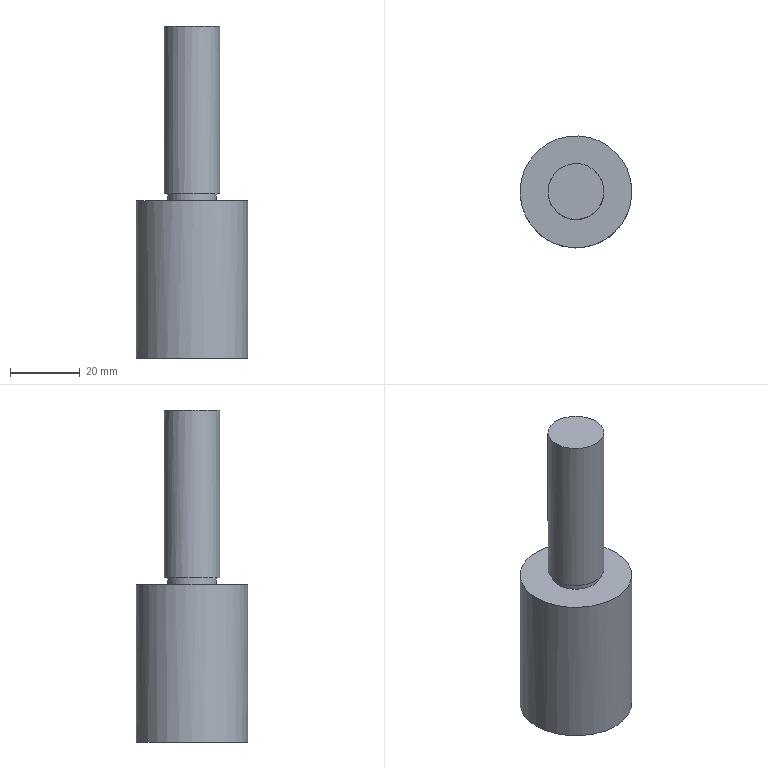Part | NX | features solid 2 | 1 solid | 9 faces | box 32 x 32 x 95 mm | volume 42869 mm3 | cylinder 4 | plane 3 | spline 2 | commonest cylinder face diameters 12 x1 14 x1 16 x1 32 x1
STEP:
#1=CARTESIAN_POINT('',(339.602,-73.46,-40.));
#2=VERTEX_POINT('',#1);
#3=CARTESIAN_POINT('',(336.254,-68.05,-40.));
#4=CARTESIAN_POINT('',(341.244,-75.038,-40.));
#5=CARTESIAN_POINT('',(341.565,-86.314,-40.));
#6=CARTESIAN_POINT('',(332.258,-96.177,-40.));
#7=CARTESIAN_POINT('',(318.691,-96.572,-40.));
#8=CARTESIAN_POINT('',(308.82,-87.251,-40.));
#9=CARTESIAN_POINT('',(308.429,-73.695,-40.));
#10=CARTESIAN_POINT('',(316.18,-65.49,-40.));
#11=CARTESIAN_POINT('',(324.525,-63.592,-40.));
#12=CARTESIAN_POINT('',(330.839,-64.658,-40.));
#13=CARTESIAN_POINT('',(336.254,-68.05,-40.));
#14=CARTESIAN_POINT('',(341.244,-75.038,-40.));
#15=CARTESIAN_POINT('',(341.565,-86.314,-40.));
#16=B_SPLINE_CURVE_WITH_KNOTS('',3,(#3,#4,#5,#6,#7,#8,#9,#10,#11,#12,#13,#14,#15),.UNSPECIFIED.,.T.,.F.,(1,1,1,1,1,1,1,1,1,1,1,1,1,1,1,1,1),(-0.01876,-0.0125,-0.006252,0.,0.0125,0.02501,0.03751,0.05002,0.06252,0.07503,0.08128,0.08753,0.09378,0.1,0.1125,0.125,0.1375),.UNSPECIFIED.);
#17=EDGE_CURVE('',#2,#2,#16,.T.);
#18=ORIENTED_EDGE('',*,*,#17,.F.);
#19=EDGE_LOOP('',(#18));
#20=FACE_BOUND('',#19,.T.);
#21=CARTESIAN_POINT('',(331.654,-77.826,-40.));
#22=VERTEX_POINT('',#21);
#23=CARTESIAN_POINT('',(328.504,-73.078,-40.));
#24=CARTESIAN_POINT('',(332.376,-77.591,-40.));
#25=CARTESIAN_POINT('',(331.915,-83.512,-40.));
#26=CARTESIAN_POINT('',(327.414,-87.371,-40.));
#27=CARTESIAN_POINT('',(321.493,-86.921,-40.));
#28=CARTESIAN_POINT('',(317.627,-82.41,-40.));
#29=CARTESIAN_POINT('',(318.079,-76.498,-40.));
#30=CARTESIAN_POINT('',(322.583,-72.629,-40.));
#31=CARTESIAN_POINT('',(328.504,-73.078,-40.));
#32=CARTESIAN_POINT('',(332.376,-77.591,-40.));
#33=CARTESIAN_POINT('',(331.915,-83.512,-40.));
#34=B_SPLINE_CURVE_WITH_KNOTS('',3,(#23,#24,#25,#26,#27,#28,#29,#30,#31,#32,#33),.UNSPECIFIED.,.T.,.F.,(1,1,1,1,1,1,1,1,1,1,1,1,1,1,1),(-0.01641,-0.01094,-0.005471,0.,0.005471,0.01094,0.01641,0.02188,0.02735,0.03282,0.03829,0.04377,0.04924,0.05471,0.06018),.UNSPECIFIED.);
#35=EDGE_CURVE('',#22,#22,#34,.T.);
#36=ORIENTED_EDGE('',*,*,#35,.T.);
#37=EDGE_LOOP('',(#36));
#38=FACE_BOUND('',#37,.T.);
#39=CARTESIAN_POINT('',(341.192,-96.192,-40.));
#40=CARTESIAN_POINT('',(341.192,-85.397,-40.));
#41=CARTESIAN_POINT('',(341.192,-74.603,-40.));
#42=CARTESIAN_POINT('',(341.192,-63.808,-40.));
#43=CARTESIAN_POINT('',(330.397,-96.192,-40.));
#44=CARTESIAN_POINT('',(330.397,-85.397,-40.));
#45=CARTESIAN_POINT('',(330.397,-74.603,-40.));
#46=CARTESIAN_POINT('',(330.397,-63.808,-40.));
#47=CARTESIAN_POINT('',(319.603,-96.192,-40.));
#48=CARTESIAN_POINT('',(319.603,-85.397,-40.));
#49=CARTESIAN_POINT('',(319.603,-74.603,-40.));
#50=CARTESIAN_POINT('',(319.603,-63.808,-40.));
#51=CARTESIAN_POINT('',(308.808,-96.192,-40.));
#52=CARTESIAN_POINT('',(308.808,-85.397,-40.));
#53=CARTESIAN_POINT('',(308.808,-74.603,-40.));
#54=CARTESIAN_POINT('',(308.808,-63.808,-40.));
#55=B_SPLINE_SURFACE_WITH_KNOTS('',3,3,((#39,#40,#41,#42),(#43,#44,#45,#46),(#47,#48,#49,#50),(#51,#52,#53,#54)),.UNSPECIFIED.,.F.,.F.,.F.,(4,4),(4,4),(0.,1.),(0.,1.),.UNSPECIFIED.);
#56=ADVANCED_FACE('',(#20,#38),#55,.F.);
#57=CARTESIAN_POINT('',(309.,-80.,-85.));
#58=VERTEX_POINT('',#57);
#59=CARTESIAN_POINT('',(325.,-80.,-85.));
#60=DIRECTION('',(0.,0.,-1.));
#61=DIRECTION('',(-1.,0.,0.));
#62=AXIS2_PLACEMENT_3D('',#59,#60,#61);
#63=CIRCLE('',#62,16.);
#64=EDGE_CURVE('',#58,#58,#63,.T.);
#65=ORIENTED_EDGE('',*,*,#64,.F.);
#66=EDGE_LOOP('',(#65));
#67=FACE_BOUND('',#66,.T.);
#68=ORIENTED_EDGE('',*,*,#17,.T.);
#69=EDGE_LOOP('',(#68));
#70=FACE_BOUND('',#69,.T.);
#71=CARTESIAN_POINT('',(325.,-80.,-7.));
#72=DIRECTION('',(0.,0.,-1.));
#73=DIRECTION('',(1.,0.,0.));
#74=AXIS2_PLACEMENT_3D('',#71,#72,#73);
#75=CYLINDRICAL_SURFACE('',#74,16.);
#76=ADVANCED_FACE('',(#67,#70),#75,.T.);
#77=ORIENTED_EDGE('',*,*,#64,.T.);
#78=EDGE_LOOP('',(#77));
#79=FACE_BOUND('',#78,.T.);
#80=CARTESIAN_POINT('',(319.,-80.,-85.));
#81=VERTEX_POINT('',#80);
#82=CARTESIAN_POINT('',(325.,-80.,-85.));
#83=DIRECTION('',(0.,0.,-1.));
#84=DIRECTION('',(-1.,0.,0.));
#85=AXIS2_PLACEMENT_3D('',#82,#83,#84);
#86=CIRCLE('',#85,6.);
#87=EDGE_CURVE('',#81,#81,#86,.T.);
#88=ORIENTED_EDGE('',*,*,#87,.F.);
#89=EDGE_LOOP('',(#88));
#90=FACE_BOUND('',#89,.T.);
#91=CARTESIAN_POINT('',(325.,-80.,-85.));
#92=DIRECTION('',(0.,0.,1.));
#93=DIRECTION('',(-1.,0.,0.));
#94=AXIS2_PLACEMENT_3D('',#91,#92,#93);
#95=PLANE('',#94);
#96=ADVANCED_FACE('',(#79,#90),#95,.F.);
#97=CARTESIAN_POINT('',(319.,-80.,-56.));
#98=VERTEX_POINT('',#97);
#99=CARTESIAN_POINT('',(325.,-80.,-56.));
#100=DIRECTION('',(0.,0.,-1.));
#101=DIRECTION('',(-1.,0.,0.));
#102=AXIS2_PLACEMENT_3D('',#99,#100,#101);
#103=CIRCLE('',#102,6.);
#104=EDGE_CURVE('',#98,#98,#103,.T.);
#105=ORIENTED_EDGE('',*,*,#104,.T.);
#106=EDGE_LOOP('',(#105));
#107=FACE_BOUND('',#106,.T.);
#108=CARTESIAN_POINT('',(325.,-80.,-56.));
#109=DIRECTION('',(0.,0.,1.));
#110=DIRECTION('',(1.,0.,0.));
#111=AXIS2_PLACEMENT_3D('',#108,#109,#110);
#112=PLANE('',#111);
#113=ADVANCED_FACE('',(#107),#112,.F.);
#114=ORIENTED_EDGE('',*,*,#87,.T.);
#115=EDGE_LOOP('',(#114));
#116=FACE_BOUND('',#115,.T.);
#117=ORIENTED_EDGE('',*,*,#104,.F.);
#118=EDGE_LOOP('',(#117));
#119=FACE_BOUND('',#118,.T.);
#120=CARTESIAN_POINT('',(325.,-80.,-86.));
#121=DIRECTION('',(0.,0.,-1.));
#122=DIRECTION('',(-1.,0.,0.));
#123=AXIS2_PLACEMENT_3D('',#120,#121,#122);
#124=CYLINDRICAL_SURFACE('',#123,6.);
#125=ADVANCED_FACE('',(#116,#119),#124,.F.);
#126=ORIENTED_EDGE('',*,*,#35,.F.);
#127=EDGE_LOOP('',(#126));
#128=FACE_BOUND('',#127,.T.);
#129=CARTESIAN_POINT('',(331.389,-77.139,-38.));
#130=VERTEX_POINT('',#129);
#131=CARTESIAN_POINT('',(327.758,-72.748,-38.));
#132=CARTESIAN_POINT('',(332.082,-76.83,-38.));
#133=CARTESIAN_POINT('',(332.246,-82.766,-38.));
#134=CARTESIAN_POINT('',(328.176,-87.076,-38.));
#135=CARTESIAN_POINT('',(322.24,-87.251,-38.));
#136=CARTESIAN_POINT('',(317.921,-83.171,-38.));
#137=CARTESIAN_POINT('',(317.75,-77.245,-38.));
#138=CARTESIAN_POINT('',(321.822,-72.924,-38.));
#139=CARTESIAN_POINT('',(327.758,-72.748,-38.));
#140=CARTESIAN_POINT('',(332.082,-76.83,-38.));
#141=CARTESIAN_POINT('',(332.246,-82.766,-38.));
#142=B_SPLINE_CURVE_WITH_KNOTS('',3,(#131,#132,#133,#134,#135,#136,#137,#138,#139,#140,#141),.UNSPECIFIED.,.T.,.F.,(1,1,1,1,1,1,1,1,1,1,1,1,1,1,1),(-0.01641,-0.01094,-0.005471,0.,0.005471,0.01094,0.01641,0.02188,0.02735,0.03282,0.03829,0.04377,0.04924,0.05471,0.06018),.UNSPECIFIED.);
#143=EDGE_CURVE('',#130,#130,#142,.T.);
#144=ORIENTED_EDGE('',*,*,#143,.T.);
#145=EDGE_LOOP('',(#144));
#146=FACE_BOUND('',#145,.T.);
#147=CARTESIAN_POINT('',(325.,-80.,-7.));
#148=DIRECTION('',(0.,0.,-1.));
#149=DIRECTION('',(1.,0.,0.));
#150=AXIS2_PLACEMENT_3D('',#147,#148,#149);
#151=CYLINDRICAL_SURFACE('',#150,7.);
#152=ADVANCED_FACE('',(#128,#146),#151,.T.);
#153=CARTESIAN_POINT('',(317.396,-82.485,-38.));
#154=VERTEX_POINT('',#153);
#155=CARTESIAN_POINT('',(320.995,-87.911,-38.));
#156=CARTESIAN_POINT('',(316.571,-82.753,-38.));
#157=CARTESIAN_POINT('',(317.097,-75.987,-38.));
#158=CARTESIAN_POINT('',(322.241,-71.576,-38.));
#159=CARTESIAN_POINT('',(329.008,-72.091,-38.));
#160=CARTESIAN_POINT('',(333.426,-77.246,-38.));
#161=CARTESIAN_POINT('',(332.909,-84.002,-38.));
#162=CARTESIAN_POINT('',(327.763,-88.424,-38.));
#163=CARTESIAN_POINT('',(320.995,-87.911,-38.));
#164=CARTESIAN_POINT('',(316.571,-82.753,-38.));
#165=CARTESIAN_POINT('',(317.097,-75.987,-38.));
#166=B_SPLINE_CURVE_WITH_KNOTS('',3,(#155,#156,#157,#158,#159,#160,#161,#162,#163,#164,#165),.UNSPECIFIED.,.T.,.F.,(1,1,1,1,1,1,1,1,1,1,1,1,1,1,1),(-0.01876,-0.0125,-0.006252,0.,0.006252,0.0125,0.01876,0.02501,0.03126,0.03751,0.04377,0.05002,0.05627,0.06252,0.06877),.UNSPECIFIED.);
#167=EDGE_CURVE('',#154,#154,#166,.T.);
#168=ORIENTED_EDGE('',*,*,#167,.T.);
#169=EDGE_LOOP('',(#168));
#170=FACE_BOUND('',#169,.T.);
#171=ORIENTED_EDGE('',*,*,#143,.F.);
#172=EDGE_LOOP('',(#171));
#173=FACE_BOUND('',#172,.T.);
#174=CARTESIAN_POINT('',(333.143,-88.121,-38.));
#175=CARTESIAN_POINT('',(333.143,-82.7,-38.));
#176=CARTESIAN_POINT('',(333.143,-77.278,-38.));
#177=CARTESIAN_POINT('',(333.143,-71.856,-38.));
#178=CARTESIAN_POINT('',(327.724,-88.121,-38.));
#179=CARTESIAN_POINT('',(327.724,-82.7,-38.));
#180=CARTESIAN_POINT('',(327.724,-77.278,-38.));
#181=CARTESIAN_POINT('',(327.724,-71.856,-38.));
#182=CARTESIAN_POINT('',(322.305,-88.121,-38.));
#183=CARTESIAN_POINT('',(322.305,-82.7,-38.));
#184=CARTESIAN_POINT('',(322.305,-77.278,-38.));
#185=CARTESIAN_POINT('',(322.305,-71.856,-38.));
#186=CARTESIAN_POINT('',(316.886,-88.121,-38.));
#187=CARTESIAN_POINT('',(316.886,-82.7,-38.));
#188=CARTESIAN_POINT('',(316.886,-77.278,-38.));
#189=CARTESIAN_POINT('',(316.886,-71.856,-38.));
#190=B_SPLINE_SURFACE_WITH_KNOTS('',3,3,((#174,#175,#176,#177),(#178,#179,#180,#181),(#182,#183,#184,#185),(#186,#187,#188,#189)),.UNSPECIFIED.,.F.,.F.,.F.,(4,4),(4,4),(0.2485,0.7506),(0.2492,0.7515),.UNSPECIFIED.);
#191=ADVANCED_FACE('',(#170,#173),#190,.T.);
#192=CARTESIAN_POINT('',(317.,-80.,10.));
#193=VERTEX_POINT('',#192);
#194=CARTESIAN_POINT('',(325.,-80.,10.));
#195=DIRECTION('',(0.,0.,-1.));
#196=DIRECTION('',(-1.,0.,0.));
#197=AXIS2_PLACEMENT_3D('',#194,#195,#196);
#198=CIRCLE('',#197,8.);
#199=EDGE_CURVE('',#193,#193,#198,.T.);
#200=ORIENTED_EDGE('',*,*,#199,.F.);
#201=EDGE_LOOP('',(#200));
#202=FACE_BOUND('',#201,.T.);
#203=CARTESIAN_POINT('',(325.,-80.,10.));
#204=DIRECTION('',(0.,0.,1.));
#205=DIRECTION('',(-1.,0.,0.));
#206=AXIS2_PLACEMENT_3D('',#203,#204,#205);
#207=PLANE('',#206);
#208=ADVANCED_FACE('',(#202),#207,.T.);
#209=ORIENTED_EDGE('',*,*,#167,.F.);
#210=EDGE_LOOP('',(#209));
#211=FACE_BOUND('',#210,.T.);
#212=ORIENTED_EDGE('',*,*,#199,.T.);
#213=EDGE_LOOP('',(#212));
#214=FACE_BOUND('',#213,.T.);
#215=CARTESIAN_POINT('',(325.,-80.,-7.));
#216=DIRECTION('',(0.,0.,-1.));
#217=DIRECTION('',(1.,0.,0.));
#218=AXIS2_PLACEMENT_3D('',#215,#216,#217);
#219=CYLINDRICAL_SURFACE('',#218,8.);
#220=ADVANCED_FACE('',(#211,#214),#219,.T.);
#221=CLOSED_SHELL('',(#56,#76,#96,#113,#125,#152,#191,#208,#220));
#222=MANIFOLD_SOLID_BREP('',#221);
#223=(LENGTH_UNIT()NAMED_UNIT(*)SI_UNIT(.MILLI.,.METRE.));
#224=UNCERTAINTY_MEASURE_WITH_UNIT(LENGTH_MEASURE(0.0508),#223,'','');
#225=(NAMED_UNIT(*)PLANE_ANGLE_UNIT()SI_UNIT($,.RADIAN.));
#226=(NAMED_UNIT(*)SI_UNIT($,.STERADIAN.)SOLID_ANGLE_UNIT());
#227=(GEOMETRIC_REPRESENTATION_CONTEXT(3)GLOBAL_UNCERTAINTY_ASSIGNED_CONTEXT((#224))GLOBAL_UNIT_ASSIGNED_CONTEXT((#223,#225,#226))REPRESENTATION_CONTEXT('',''));
#228=ADVANCED_BREP_SHAPE_REPRESENTATION('',(#222),#227);